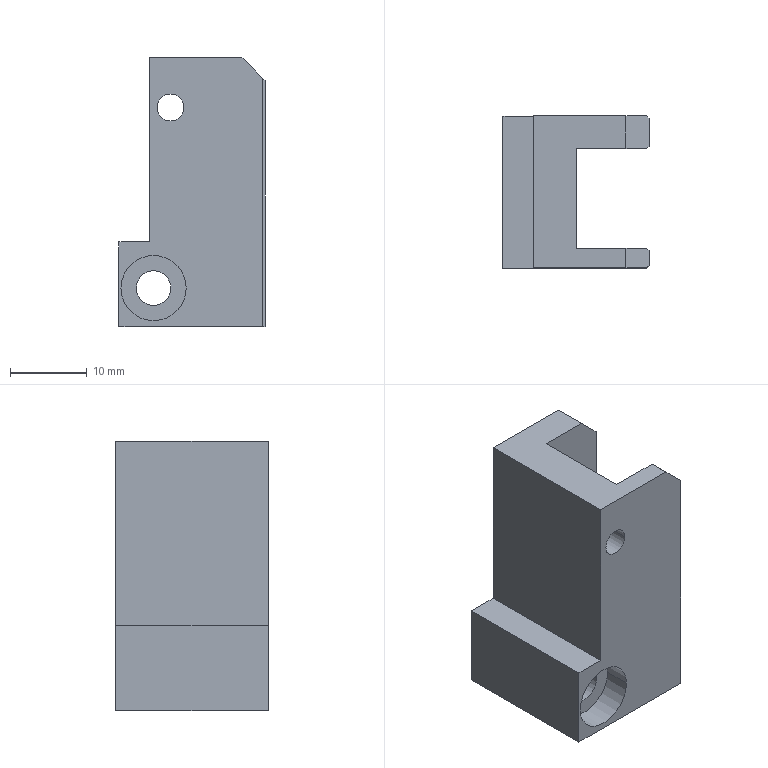Part | NX | 1 solid | 25 faces | box 19 x 19.788 x 35 mm | volume 6253 mm3 | plane 19 | cylinder 6 | commonest cylinder face diameters 3.5 x2 4.5 x2 8.5 x2
STEP:
#1=CARTESIAN_POINT('',(9.5,16.462,0.));
#2=VERTEX_POINT('',#1);
#3=CARTESIAN_POINT('',(18.7,16.462,0.));
#4=VERTEX_POINT('',#3);
#5=CARTESIAN_POINT('',(0.,16.462,0.));
#6=DIRECTION('',(1.,0.,0.));
#7=VECTOR('',#6,1000.);
#8=LINE('',#5,#7);
#9=EDGE_CURVE('',#2,#4,#8,.T.);
#10=ORIENTED_EDGE('',*,*,#9,.F.);
#11=CARTESIAN_POINT('',(9.5,3.462,0.));
#12=VERTEX_POINT('',#11);
#13=CARTESIAN_POINT('',(9.5,0.,0.));
#14=DIRECTION('',(0.,1.,0.));
#15=VECTOR('',#14,1000.);
#16=LINE('',#13,#15);
#17=EDGE_CURVE('',#12,#2,#16,.T.);
#18=ORIENTED_EDGE('',*,*,#17,.F.);
#19=CARTESIAN_POINT('',(18.7,3.462,0.));
#20=VERTEX_POINT('',#19);
#21=CARTESIAN_POINT('',(0.,3.462,0.));
#22=DIRECTION('',(-1.,0.,0.));
#23=VECTOR('',#22,1000.);
#24=LINE('',#21,#23);
#25=EDGE_CURVE('',#20,#12,#24,.T.);
#26=ORIENTED_EDGE('',*,*,#25,.F.);
#27=CARTESIAN_POINT('',(19.,3.162,0.));
#28=VERTEX_POINT('',#27);
#29=CARTESIAN_POINT('',(0.,22.162,0.));
#30=DIRECTION('',(0.7071,-0.7071,0.));
#31=VECTOR('',#30,1000.);
#32=LINE('',#29,#31);
#33=EDGE_CURVE('',#20,#28,#32,.T.);
#34=ORIENTED_EDGE('',*,*,#33,.T.);
#35=CARTESIAN_POINT('',(19.,1.212,0.));
#36=VERTEX_POINT('',#35);
#37=CARTESIAN_POINT('',(19.,0.,0.));
#38=DIRECTION('',(0.,-1.,0.));
#39=VECTOR('',#38,1000.);
#40=LINE('',#37,#39);
#41=EDGE_CURVE('',#28,#36,#40,.T.);
#42=ORIENTED_EDGE('',*,*,#41,.T.);
#43=CARTESIAN_POINT('',(18.7,0.912,0.));
#44=VERTEX_POINT('',#43);
#45=CARTESIAN_POINT('',(0.,-17.788,0.));
#46=DIRECTION('',(0.7071,0.7071,0.));
#47=VECTOR('',#46,1000.);
#48=LINE('',#45,#47);
#49=EDGE_CURVE('',#44,#36,#48,.T.);
#50=ORIENTED_EDGE('',*,*,#49,.F.);
#51=CARTESIAN_POINT('',(0.,0.912,0.));
#52=VERTEX_POINT('',#51);
#53=CARTESIAN_POINT('',(0.,0.912,0.));
#54=DIRECTION('',(-1.,0.,0.));
#55=VECTOR('',#54,1000.);
#56=LINE('',#53,#55);
#57=EDGE_CURVE('',#44,#52,#56,.T.);
#58=ORIENTED_EDGE('',*,*,#57,.T.);
#59=CARTESIAN_POINT('',(0.,20.7,0.));
#60=VERTEX_POINT('',#59);
#61=CARTESIAN_POINT('',(0.,0.,0.));
#62=DIRECTION('',(0.,-1.,0.));
#63=VECTOR('',#62,1000.);
#64=LINE('',#61,#63);
#65=EDGE_CURVE('',#60,#52,#64,.T.);
#66=ORIENTED_EDGE('',*,*,#65,.F.);
#67=CARTESIAN_POINT('',(18.7,20.7,0.));
#68=VERTEX_POINT('',#67);
#69=CARTESIAN_POINT('',(0.,20.7,0.));
#70=DIRECTION('',(1.,0.,0.));
#71=VECTOR('',#70,1000.);
#72=LINE('',#69,#71);
#73=EDGE_CURVE('',#60,#68,#72,.T.);
#74=ORIENTED_EDGE('',*,*,#73,.T.);
#75=CARTESIAN_POINT('',(19.,20.4,0.));
#76=VERTEX_POINT('',#75);
#77=CARTESIAN_POINT('',(39.4,0.,0.));
#78=DIRECTION('',(0.7071,-0.7071,0.));
#79=VECTOR('',#78,1000.);
#80=LINE('',#77,#79);
#81=EDGE_CURVE('',#68,#76,#80,.T.);
#82=ORIENTED_EDGE('',*,*,#81,.T.);
#83=CARTESIAN_POINT('',(19.,16.762,0.));
#84=VERTEX_POINT('',#83);
#85=CARTESIAN_POINT('',(19.,0.,0.));
#86=DIRECTION('',(0.,1.,0.));
#87=VECTOR('',#86,1000.);
#88=LINE('',#85,#87);
#89=EDGE_CURVE('',#84,#76,#88,.T.);
#90=ORIENTED_EDGE('',*,*,#89,.F.);
#91=CARTESIAN_POINT('',(2.238,0.,0.));
#92=DIRECTION('',(0.7071,0.7071,0.));
#93=VECTOR('',#92,1000.);
#94=LINE('',#91,#93);
#95=EDGE_CURVE('',#4,#84,#94,.T.);
#96=ORIENTED_EDGE('',*,*,#95,.F.);
#97=EDGE_LOOP('',(#10,#18,#26,#34,#42,#50,#58,#66,#74,#82,#90,#96));
#98=FACE_BOUND('',#97,.T.);
#99=CARTESIAN_POINT('',(0.,0.,0.));
#100=DIRECTION('',(0.,0.,1.));
#101=DIRECTION('',(1.,0.,0.));
#102=AXIS2_PLACEMENT_3D('',#99,#100,#101);
#103=PLANE('',#102);
#104=ADVANCED_FACE('',(#98),#103,.F.);
#105=CARTESIAN_POINT('',(18.7,16.462,32.3));
#106=VERTEX_POINT('',#105);
#107=CARTESIAN_POINT('',(18.7,16.462,0.));
#108=DIRECTION('',(0.,0.,-1.));
#109=VECTOR('',#108,1000.);
#110=LINE('',#107,#109);
#111=EDGE_CURVE('',#106,#4,#110,.T.);
#112=ORIENTED_EDGE('',*,*,#111,.F.);
#113=CARTESIAN_POINT('',(16.,16.462,35.));
#114=VERTEX_POINT('',#113);
#115=CARTESIAN_POINT('',(51.,16.462,0.));
#116=DIRECTION('',(-0.7071,0.,0.7071));
#117=VECTOR('',#116,1000.);
#118=LINE('',#115,#117);
#119=EDGE_CURVE('',#106,#114,#118,.T.);
#120=ORIENTED_EDGE('',*,*,#119,.T.);
#121=CARTESIAN_POINT('',(9.5,16.462,35.));
#122=VERTEX_POINT('',#121);
#123=CARTESIAN_POINT('',(0.,16.462,35.));
#124=DIRECTION('',(1.,0.,0.));
#125=VECTOR('',#124,1000.);
#126=LINE('',#123,#125);
#127=EDGE_CURVE('',#122,#114,#126,.T.);
#128=ORIENTED_EDGE('',*,*,#127,.F.);
#129=CARTESIAN_POINT('',(9.5,16.462,0.));
#130=DIRECTION('',(0.,0.,1.));
#131=VECTOR('',#130,1000.);
#132=LINE('',#129,#131);
#133=EDGE_CURVE('',#2,#122,#132,.T.);
#134=ORIENTED_EDGE('',*,*,#133,.F.);
#135=ORIENTED_EDGE('',*,*,#9,.T.);
#136=EDGE_LOOP('',(#112,#120,#128,#134,#135));
#137=FACE_BOUND('',#136,.T.);
#138=CARTESIAN_POINT('',(19.,16.462,35.));
#139=DIRECTION('',(0.,1.,0.));
#140=DIRECTION('',(1.,0.,0.));
#141=AXIS2_PLACEMENT_3D('',#138,#139,#140);
#142=PLANE('',#141);
#143=ADVANCED_FACE('',(#137),#142,.F.);
#144=ORIENTED_EDGE('',*,*,#17,.T.);
#145=ORIENTED_EDGE('',*,*,#133,.T.);
#146=CARTESIAN_POINT('',(9.5,3.462,35.));
#147=VERTEX_POINT('',#146);
#148=CARTESIAN_POINT('',(9.5,0.,35.));
#149=DIRECTION('',(0.,1.,0.));
#150=VECTOR('',#149,1000.);
#151=LINE('',#148,#150);
#152=EDGE_CURVE('',#147,#122,#151,.T.);
#153=ORIENTED_EDGE('',*,*,#152,.F.);
#154=CARTESIAN_POINT('',(9.5,3.462,0.));
#155=DIRECTION('',(0.,0.,1.));
#156=VECTOR('',#155,1000.);
#157=LINE('',#154,#156);
#158=EDGE_CURVE('',#12,#147,#157,.T.);
#159=ORIENTED_EDGE('',*,*,#158,.F.);
#160=EDGE_LOOP('',(#144,#145,#153,#159));
#161=FACE_BOUND('',#160,.T.);
#162=CARTESIAN_POINT('',(9.5,16.95,35.));
#163=DIRECTION('',(-1.,0.,0.));
#164=DIRECTION('',(0.,0.,1.));
#165=AXIS2_PLACEMENT_3D('',#162,#163,#164);
#166=PLANE('',#165);
#167=ADVANCED_FACE('',(#161),#166,.F.);
#168=CARTESIAN_POINT('',(18.7,3.462,32.3));
#169=VERTEX_POINT('',#168);
#170=CARTESIAN_POINT('',(18.7,3.462,0.));
#171=DIRECTION('',(0.,0.,-1.));
#172=VECTOR('',#171,1000.);
#173=LINE('',#170,#172);
#174=EDGE_CURVE('',#169,#20,#173,.T.);
#175=ORIENTED_EDGE('',*,*,#174,.T.);
#176=ORIENTED_EDGE('',*,*,#25,.T.);
#177=ORIENTED_EDGE('',*,*,#158,.T.);
#178=CARTESIAN_POINT('',(16.,3.462,35.));
#179=VERTEX_POINT('',#178);
#180=CARTESIAN_POINT('',(0.,3.462,35.));
#181=DIRECTION('',(-1.,0.,0.));
#182=VECTOR('',#181,1000.);
#183=LINE('',#180,#182);
#184=EDGE_CURVE('',#179,#147,#183,.T.);
#185=ORIENTED_EDGE('',*,*,#184,.F.);
#186=CARTESIAN_POINT('',(51.,3.462,0.));
#187=DIRECTION('',(0.7071,0.,-0.7071));
#188=VECTOR('',#187,1000.);
#189=LINE('',#186,#188);
#190=EDGE_CURVE('',#179,#169,#189,.T.);
#191=ORIENTED_EDGE('',*,*,#190,.T.);
#192=EDGE_LOOP('',(#175,#176,#177,#185,#191));
#193=FACE_BOUND('',#192,.T.);
#194=CARTESIAN_POINT('',(9.5,3.462,35.));
#195=DIRECTION('',(0.,-1.,0.));
#196=DIRECTION('',(0.,0.,-1.));
#197=AXIS2_PLACEMENT_3D('',#194,#195,#196);
#198=PLANE('',#197);
#199=ADVANCED_FACE('',(#193),#198,.F.);
#200=CARTESIAN_POINT('',(19.,3.162,32.));
#201=VERTEX_POINT('',#200);
#202=CARTESIAN_POINT('',(19.,3.162,0.));
#203=DIRECTION('',(0.,0.,-1.));
#204=VECTOR('',#203,1000.);
#205=LINE('',#202,#204);
#206=EDGE_CURVE('',#201,#28,#205,.T.);
#207=ORIENTED_EDGE('',*,*,#206,.F.);
#208=CARTESIAN_POINT('',(19.,1.212,32.));
#209=VERTEX_POINT('',#208);
#210=CARTESIAN_POINT('',(19.,0.,32.));
#211=DIRECTION('',(0.,1.,0.));
#212=VECTOR('',#211,1000.);
#213=LINE('',#210,#212);
#214=EDGE_CURVE('',#209,#201,#213,.T.);
#215=ORIENTED_EDGE('',*,*,#214,.F.);
#216=CARTESIAN_POINT('',(19.,1.212,0.));
#217=DIRECTION('',(0.,0.,-1.));
#218=VECTOR('',#217,1000.);
#219=LINE('',#216,#218);
#220=EDGE_CURVE('',#209,#36,#219,.T.);
#221=ORIENTED_EDGE('',*,*,#220,.T.);
#222=ORIENTED_EDGE('',*,*,#41,.F.);
#223=EDGE_LOOP('',(#207,#215,#221,#222));
#224=FACE_BOUND('',#223,.T.);
#225=CARTESIAN_POINT('',(19.,0.,0.));
#226=DIRECTION('',(1.,0.,0.));
#227=DIRECTION('',(0.,1.,0.));
#228=AXIS2_PLACEMENT_3D('',#225,#226,#227);
#229=PLANE('',#228);
#230=ADVANCED_FACE('',(#224),#229,.T.);
#231=CARTESIAN_POINT('',(0.25,4.4,5.));
#232=VERTEX_POINT('',#231);
#233=CARTESIAN_POINT('',(8.75,4.4,5.));
#234=VERTEX_POINT('',#233);
#235=CARTESIAN_POINT('',(4.5,4.4,5.));
#236=DIRECTION('',(0.,-1.,0.));
#237=DIRECTION('',(-1.,0.,0.));
#238=AXIS2_PLACEMENT_3D('',#235,#236,#237);
#239=CIRCLE('',#238,4.25);
#240=EDGE_CURVE('',#232,#234,#239,.T.);
#241=ORIENTED_EDGE('',*,*,#240,.T.);
#242=CARTESIAN_POINT('',(4.5,4.4,5.));
#243=DIRECTION('',(0.,-1.,0.));
#244=DIRECTION('',(-1.,0.,0.));
#245=AXIS2_PLACEMENT_3D('',#242,#243,#244);
#246=CIRCLE('',#245,4.25);
#247=EDGE_CURVE('',#234,#232,#246,.T.);
#248=ORIENTED_EDGE('',*,*,#247,.T.);
#249=EDGE_LOOP('',(#241,#248));
#250=FACE_BOUND('',#249,.T.);
#251=CARTESIAN_POINT('',(2.25,4.4,5.));
#252=VERTEX_POINT('',#251);
#253=CARTESIAN_POINT('',(6.75,4.4,5.));
#254=VERTEX_POINT('',#253);
#255=CARTESIAN_POINT('',(4.5,4.4,5.));
#256=DIRECTION('',(0.,-1.,0.));
#257=DIRECTION('',(1.,0.,0.));
#258=AXIS2_PLACEMENT_3D('',#255,#256,#257);
#259=CIRCLE('',#258,2.25);
#260=EDGE_CURVE('',#252,#254,#259,.T.);
#261=ORIENTED_EDGE('',*,*,#260,.F.);
#262=CARTESIAN_POINT('',(4.5,4.4,5.));
#263=DIRECTION('',(0.,-1.,0.));
#264=DIRECTION('',(1.,0.,0.));
#265=AXIS2_PLACEMENT_3D('',#262,#263,#264);
#266=CIRCLE('',#265,2.25);
#267=EDGE_CURVE('',#254,#252,#266,.T.);
#268=ORIENTED_EDGE('',*,*,#267,.F.);
#269=EDGE_LOOP('',(#261,#268));
#270=FACE_BOUND('',#269,.T.);
#271=CARTESIAN_POINT('',(9.199,4.4,2.964));
#272=DIRECTION('',(0.,-1.,0.));
#273=DIRECTION('',(0.,0.,-1.));
#274=AXIS2_PLACEMENT_3D('',#271,#272,#273);
#275=PLANE('',#274);
#276=ADVANCED_FACE('',(#250,#270),#275,.T.);
#277=CARTESIAN_POINT('',(4.,20.7,35.));
#278=VERTEX_POINT('',#277);
#279=CARTESIAN_POINT('',(4.,0.912,35.));
#280=VERTEX_POINT('',#279);
#281=CARTESIAN_POINT('',(4.,0.,35.));
#282=DIRECTION('',(0.,-1.,0.));
#283=VECTOR('',#282,1000.);
#284=LINE('',#281,#283);
#285=EDGE_CURVE('',#278,#280,#284,.T.);
#286=ORIENTED_EDGE('',*,*,#285,.F.);
#287=CARTESIAN_POINT('',(4.,20.7,11.));
#288=VERTEX_POINT('',#287);
#289=CARTESIAN_POINT('',(4.,20.7,0.));
#290=DIRECTION('',(0.,0.,-1.));
#291=VECTOR('',#290,1000.);
#292=LINE('',#289,#291);
#293=EDGE_CURVE('',#278,#288,#292,.T.);
#294=ORIENTED_EDGE('',*,*,#293,.T.);
#295=CARTESIAN_POINT('',(4.,0.912,11.));
#296=VERTEX_POINT('',#295);
#297=CARTESIAN_POINT('',(4.,0.,11.));
#298=DIRECTION('',(0.,1.,0.));
#299=VECTOR('',#298,1000.);
#300=LINE('',#297,#299);
#301=EDGE_CURVE('',#296,#288,#300,.T.);
#302=ORIENTED_EDGE('',*,*,#301,.F.);
#303=CARTESIAN_POINT('',(4.,0.912,0.));
#304=DIRECTION('',(0.,0.,1.));
#305=VECTOR('',#304,1000.);
#306=LINE('',#303,#305);
#307=EDGE_CURVE('',#296,#280,#306,.T.);
#308=ORIENTED_EDGE('',*,*,#307,.T.);
#309=EDGE_LOOP('',(#286,#294,#302,#308));
#310=FACE_BOUND('',#309,.T.);
#311=CARTESIAN_POINT('',(4.,20.5,35.));
#312=DIRECTION('',(1.,0.,0.));
#313=DIRECTION('',(0.,1.,0.));
#314=AXIS2_PLACEMENT_3D('',#311,#312,#313);
#315=PLANE('',#314);
#316=ADVANCED_FACE('',(#310),#315,.F.);
#317=ORIENTED_EDGE('',*,*,#285,.T.);
#318=CARTESIAN_POINT('',(16.,0.912,35.));
#319=VERTEX_POINT('',#318);
#320=CARTESIAN_POINT('',(0.,0.912,35.));
#321=DIRECTION('',(-1.,0.,0.));
#322=VECTOR('',#321,1000.);
#323=LINE('',#320,#322);
#324=EDGE_CURVE('',#319,#280,#323,.T.);
#325=ORIENTED_EDGE('',*,*,#324,.F.);
#326=CARTESIAN_POINT('',(16.,0.,35.));
#327=DIRECTION('',(0.,1.,0.));
#328=VECTOR('',#327,1000.);
#329=LINE('',#326,#328);
#330=EDGE_CURVE('',#319,#179,#329,.T.);
#331=ORIENTED_EDGE('',*,*,#330,.T.);
#332=ORIENTED_EDGE('',*,*,#184,.T.);
#333=ORIENTED_EDGE('',*,*,#152,.T.);
#334=ORIENTED_EDGE('',*,*,#127,.T.);
#335=CARTESIAN_POINT('',(16.,20.7,35.));
#336=VERTEX_POINT('',#335);
#337=CARTESIAN_POINT('',(16.,0.,35.));
#338=DIRECTION('',(0.,-1.,0.));
#339=VECTOR('',#338,1000.);
#340=LINE('',#337,#339);
#341=EDGE_CURVE('',#336,#114,#340,.T.);
#342=ORIENTED_EDGE('',*,*,#341,.F.);
#343=CARTESIAN_POINT('',(0.,20.7,35.));
#344=DIRECTION('',(1.,0.,0.));
#345=VECTOR('',#344,1000.);
#346=LINE('',#343,#345);
#347=EDGE_CURVE('',#278,#336,#346,.T.);
#348=ORIENTED_EDGE('',*,*,#347,.F.);
#349=EDGE_LOOP('',(#317,#325,#331,#332,#333,#334,#342,#348));
#350=FACE_BOUND('',#349,.T.);
#351=CARTESIAN_POINT('',(0.,0.,35.));
#352=DIRECTION('',(0.,0.,1.));
#353=DIRECTION('',(1.,0.,0.));
#354=AXIS2_PLACEMENT_3D('',#351,#352,#353);
#355=PLANE('',#354);
#356=ADVANCED_FACE('',(#350),#355,.T.);
#357=CARTESIAN_POINT('',(18.7,0.912,32.3));
#358=VERTEX_POINT('',#357);
#359=CARTESIAN_POINT('',(18.7,0.912,0.));
#360=DIRECTION('',(0.,0.,1.));
#361=VECTOR('',#360,1000.);
#362=LINE('',#359,#361);
#363=EDGE_CURVE('',#44,#358,#362,.T.);
#364=ORIENTED_EDGE('',*,*,#363,.T.);
#365=CARTESIAN_POINT('',(51.,0.912,0.));
#366=DIRECTION('',(0.7071,0.,-0.7071));
#367=VECTOR('',#366,1000.);
#368=LINE('',#365,#367);
#369=EDGE_CURVE('',#319,#358,#368,.T.);
#370=ORIENTED_EDGE('',*,*,#369,.F.);
#371=ORIENTED_EDGE('',*,*,#324,.T.);
#372=ORIENTED_EDGE('',*,*,#307,.F.);
#373=CARTESIAN_POINT('',(0.,0.912,11.));
#374=VERTEX_POINT('',#373);
#375=CARTESIAN_POINT('',(0.,0.912,11.));
#376=DIRECTION('',(1.,0.,0.));
#377=VECTOR('',#376,1000.);
#378=LINE('',#375,#377);
#379=EDGE_CURVE('',#374,#296,#378,.T.);
#380=ORIENTED_EDGE('',*,*,#379,.F.);
#381=CARTESIAN_POINT('',(0.,0.912,0.));
#382=DIRECTION('',(0.,0.,-1.));
#383=VECTOR('',#382,1000.);
#384=LINE('',#381,#383);
#385=EDGE_CURVE('',#374,#52,#384,.T.);
#386=ORIENTED_EDGE('',*,*,#385,.T.);
#387=ORIENTED_EDGE('',*,*,#57,.F.);
#388=EDGE_LOOP('',(#364,#370,#371,#372,#380,#386,#387));
#389=FACE_BOUND('',#388,.T.);
#390=CARTESIAN_POINT('',(8.45,0.912,28.5));
#391=VERTEX_POINT('',#390);
#392=CARTESIAN_POINT('',(4.95,0.912,28.5));
#393=VERTEX_POINT('',#392);
#394=CARTESIAN_POINT('',(6.7,0.912,28.5));
#395=DIRECTION('',(0.,-1.,0.));
#396=DIRECTION('',(1.,0.,0.));
#397=AXIS2_PLACEMENT_3D('',#394,#395,#396);
#398=CIRCLE('',#397,1.75);
#399=EDGE_CURVE('',#391,#393,#398,.T.);
#400=ORIENTED_EDGE('',*,*,#399,.F.);
#401=CARTESIAN_POINT('',(6.7,0.912,28.5));
#402=DIRECTION('',(0.,-1.,0.));
#403=DIRECTION('',(1.,0.,0.));
#404=AXIS2_PLACEMENT_3D('',#401,#402,#403);
#405=CIRCLE('',#404,1.75);
#406=EDGE_CURVE('',#393,#391,#405,.T.);
#407=ORIENTED_EDGE('',*,*,#406,.F.);
#408=EDGE_LOOP('',(#400,#407));
#409=FACE_BOUND('',#408,.T.);
#410=CARTESIAN_POINT('',(0.25,0.912,5.));
#411=VERTEX_POINT('',#410);
#412=CARTESIAN_POINT('',(8.75,0.912,5.));
#413=VERTEX_POINT('',#412);
#414=CARTESIAN_POINT('',(4.5,0.912,5.));
#415=DIRECTION('',(0.,-1.,0.));
#416=DIRECTION('',(-1.,0.,0.));
#417=AXIS2_PLACEMENT_3D('',#414,#415,#416);
#418=CIRCLE('',#417,4.25);
#419=EDGE_CURVE('',#411,#413,#418,.T.);
#420=ORIENTED_EDGE('',*,*,#419,.F.);
#421=CARTESIAN_POINT('',(4.5,0.912,5.));
#422=DIRECTION('',(0.,-1.,0.));
#423=DIRECTION('',(-1.,0.,0.));
#424=AXIS2_PLACEMENT_3D('',#421,#422,#423);
#425=CIRCLE('',#424,4.25);
#426=EDGE_CURVE('',#413,#411,#425,.T.);
#427=ORIENTED_EDGE('',*,*,#426,.F.);
#428=EDGE_LOOP('',(#420,#427));
#429=FACE_BOUND('',#428,.T.);
#430=CARTESIAN_POINT('',(0.,0.912,0.));
#431=DIRECTION('',(0.,-1.,0.));
#432=DIRECTION('',(0.,0.,-1.));
#433=AXIS2_PLACEMENT_3D('',#430,#431,#432);
#434=PLANE('',#433);
#435=ADVANCED_FACE('',(#389,#409,#429),#434,.T.);
#436=ORIENTED_EDGE('',*,*,#379,.T.);
#437=ORIENTED_EDGE('',*,*,#301,.T.);
#438=CARTESIAN_POINT('',(0.,20.7,11.));
#439=VERTEX_POINT('',#438);
#440=CARTESIAN_POINT('',(0.,20.7,11.));
#441=DIRECTION('',(-1.,0.,0.));
#442=VECTOR('',#441,1000.);
#443=LINE('',#440,#442);
#444=EDGE_CURVE('',#288,#439,#443,.T.);
#445=ORIENTED_EDGE('',*,*,#444,.T.);
#446=CARTESIAN_POINT('',(0.,0.,11.));
#447=DIRECTION('',(0.,-1.,0.));
#448=VECTOR('',#447,1000.);
#449=LINE('',#446,#448);
#450=EDGE_CURVE('',#439,#374,#449,.T.);
#451=ORIENTED_EDGE('',*,*,#450,.T.);
#452=EDGE_LOOP('',(#436,#437,#445,#451));
#453=FACE_BOUND('',#452,.T.);
#454=CARTESIAN_POINT('',(4.,20.5,11.));
#455=DIRECTION('',(0.,0.,-1.));
#456=DIRECTION('',(0.,-1.,0.));
#457=AXIS2_PLACEMENT_3D('',#454,#455,#456);
#458=PLANE('',#457);
#459=ADVANCED_FACE('',(#453),#458,.F.);
#460=ORIENTED_EDGE('',*,*,#450,.F.);
#461=CARTESIAN_POINT('',(0.,20.7,0.));
#462=DIRECTION('',(0.,0.,1.));
#463=VECTOR('',#462,1000.);
#464=LINE('',#461,#463);
#465=EDGE_CURVE('',#60,#439,#464,.T.);
#466=ORIENTED_EDGE('',*,*,#465,.F.);
#467=ORIENTED_EDGE('',*,*,#65,.T.);
#468=ORIENTED_EDGE('',*,*,#385,.F.);
#469=EDGE_LOOP('',(#460,#466,#467,#468));
#470=FACE_BOUND('',#469,.T.);
#471=CARTESIAN_POINT('',(0.,20.5,0.));
#472=DIRECTION('',(-1.,0.,0.));
#473=DIRECTION('',(0.,0.,1.));
#474=AXIS2_PLACEMENT_3D('',#471,#472,#473);
#475=PLANE('',#474);
#476=ADVANCED_FACE('',(#470),#475,.T.);
#477=CARTESIAN_POINT('',(19.,16.762,32.));
#478=VERTEX_POINT('',#477);
#479=CARTESIAN_POINT('',(19.,16.762,0.));
#480=DIRECTION('',(0.,0.,-1.));
#481=VECTOR('',#480,1000.);
#482=LINE('',#479,#481);
#483=EDGE_CURVE('',#478,#84,#482,.T.);
#484=ORIENTED_EDGE('',*,*,#483,.T.);
#485=ORIENTED_EDGE('',*,*,#89,.T.);
#486=CARTESIAN_POINT('',(19.,20.4,32.));
#487=VERTEX_POINT('',#486);
#488=CARTESIAN_POINT('',(19.,20.4,0.));
#489=DIRECTION('',(0.,0.,-1.));
#490=VECTOR('',#489,1000.);
#491=LINE('',#488,#490);
#492=EDGE_CURVE('',#487,#76,#491,.T.);
#493=ORIENTED_EDGE('',*,*,#492,.F.);
#494=CARTESIAN_POINT('',(19.,0.,32.));
#495=DIRECTION('',(0.,-1.,0.));
#496=VECTOR('',#495,1000.);
#497=LINE('',#494,#496);
#498=EDGE_CURVE('',#487,#478,#497,.T.);
#499=ORIENTED_EDGE('',*,*,#498,.T.);
#500=EDGE_LOOP('',(#484,#485,#493,#499));
#501=FACE_BOUND('',#500,.T.);
#502=CARTESIAN_POINT('',(19.,0.,0.));
#503=DIRECTION('',(1.,0.,0.));
#504=DIRECTION('',(0.,1.,0.));
#505=AXIS2_PLACEMENT_3D('',#502,#503,#504);
#506=PLANE('',#505);
#507=ADVANCED_FACE('',(#501),#506,.T.);
#508=ORIENTED_EDGE('',*,*,#341,.T.);
#509=ORIENTED_EDGE('',*,*,#119,.F.);
#510=CARTESIAN_POINT('',(51.,48.762,0.));
#511=DIRECTION('',(-0.5774,-0.5774,0.5774));
#512=VECTOR('',#511,1000.);
#513=LINE('',#510,#512);
#514=EDGE_CURVE('',#478,#106,#513,.T.);
#515=ORIENTED_EDGE('',*,*,#514,.F.);
#516=ORIENTED_EDGE('',*,*,#498,.F.);
#517=CARTESIAN_POINT('',(18.7,20.7,32.3));
#518=VERTEX_POINT('',#517);
#519=CARTESIAN_POINT('',(51.,-11.6,0.));
#520=DIRECTION('',(-0.5774,0.5774,0.5774));
#521=VECTOR('',#520,1000.);
#522=LINE('',#519,#521);
#523=EDGE_CURVE('',#487,#518,#522,.T.);
#524=ORIENTED_EDGE('',*,*,#523,.T.);
#525=CARTESIAN_POINT('',(51.,20.7,0.));
#526=DIRECTION('',(-0.7071,0.,0.7071));
#527=VECTOR('',#526,1000.);
#528=LINE('',#525,#527);
#529=EDGE_CURVE('',#518,#336,#528,.T.);
#530=ORIENTED_EDGE('',*,*,#529,.T.);
#531=EDGE_LOOP('',(#508,#509,#515,#516,#524,#530));
#532=FACE_BOUND('',#531,.T.);
#533=CARTESIAN_POINT('',(16.,16.95,35.));
#534=DIRECTION('',(-0.7071,0.,-0.7071));
#535=DIRECTION('',(-0.7071,0.,0.7071));
#536=AXIS2_PLACEMENT_3D('',#533,#534,#535);
#537=PLANE('',#536);
#538=ADVANCED_FACE('',(#532),#537,.F.);
#539=CARTESIAN_POINT('',(8.45,20.7,28.5));
#540=VERTEX_POINT('',#539);
#541=CARTESIAN_POINT('',(4.95,20.7,28.5));
#542=VERTEX_POINT('',#541);
#543=CARTESIAN_POINT('',(6.7,20.7,28.5));
#544=DIRECTION('',(0.,-1.,0.));
#545=DIRECTION('',(1.,0.,0.));
#546=AXIS2_PLACEMENT_3D('',#543,#544,#545);
#547=CIRCLE('',#546,1.75);
#548=EDGE_CURVE('',#540,#542,#547,.T.);
#549=ORIENTED_EDGE('',*,*,#548,.F.);
#550=CARTESIAN_POINT('',(8.45,20.5,28.5));
#551=DIRECTION('',(0.,-1.,0.));
#552=VECTOR('',#551,1000.);
#553=LINE('',#550,#552);
#554=EDGE_CURVE('',#540,#391,#553,.T.);
#555=ORIENTED_EDGE('',*,*,#554,.T.);
#556=ORIENTED_EDGE('',*,*,#399,.T.);
#557=CARTESIAN_POINT('',(4.95,20.5,28.5));
#558=DIRECTION('',(0.,-1.,0.));
#559=VECTOR('',#558,1000.);
#560=LINE('',#557,#559);
#561=EDGE_CURVE('',#542,#393,#560,.T.);
#562=ORIENTED_EDGE('',*,*,#561,.F.);
#563=EDGE_LOOP('',(#549,#555,#556,#562));
#564=FACE_BOUND('',#563,.T.);
#565=CARTESIAN_POINT('',(6.7,20.5,28.5));
#566=DIRECTION('',(0.,-1.,0.));
#567=DIRECTION('',(1.,0.,0.));
#568=AXIS2_PLACEMENT_3D('',#565,#566,#567);
#569=CYLINDRICAL_SURFACE('',#568,1.75);
#570=ADVANCED_FACE('',(#564),#569,.F.);
#571=ORIENTED_EDGE('',*,*,#330,.F.);
#572=ORIENTED_EDGE('',*,*,#369,.T.);
#573=CARTESIAN_POINT('',(51.,33.212,0.));
#574=DIRECTION('',(-0.5774,-0.5774,0.5774));
#575=VECTOR('',#574,1000.);
#576=LINE('',#573,#575);
#577=EDGE_CURVE('',#209,#358,#576,.T.);
#578=ORIENTED_EDGE('',*,*,#577,.F.);
#579=ORIENTED_EDGE('',*,*,#214,.T.);
#580=CARTESIAN_POINT('',(51.,-28.838,0.));
#581=DIRECTION('',(-0.5774,0.5774,0.5774));
#582=VECTOR('',#581,1000.);
#583=LINE('',#580,#582);
#584=EDGE_CURVE('',#201,#169,#583,.T.);
#585=ORIENTED_EDGE('',*,*,#584,.T.);
#586=ORIENTED_EDGE('',*,*,#190,.F.);
#587=EDGE_LOOP('',(#571,#572,#578,#579,#585,#586));
#588=FACE_BOUND('',#587,.T.);
#589=CARTESIAN_POINT('',(16.,0.,35.));
#590=DIRECTION('',(-0.7071,0.,-0.7071));
#591=DIRECTION('',(-0.7071,0.,0.7071));
#592=AXIS2_PLACEMENT_3D('',#589,#590,#591);
#593=PLANE('',#592);
#594=ADVANCED_FACE('',(#588),#593,.F.);
#595=CARTESIAN_POINT('',(6.75,20.7,5.));
#596=VERTEX_POINT('',#595);
#597=CARTESIAN_POINT('',(2.25,20.7,5.));
#598=VERTEX_POINT('',#597);
#599=CARTESIAN_POINT('',(4.5,20.7,5.));
#600=DIRECTION('',(0.,-1.,0.));
#601=DIRECTION('',(1.,0.,0.));
#602=AXIS2_PLACEMENT_3D('',#599,#600,#601);
#603=CIRCLE('',#602,2.25);
#604=EDGE_CURVE('',#596,#598,#603,.T.);
#605=ORIENTED_EDGE('',*,*,#604,.F.);
#606=CARTESIAN_POINT('',(6.75,20.5,5.));
#607=DIRECTION('',(0.,-1.,0.));
#608=VECTOR('',#607,1000.);
#609=LINE('',#606,#608);
#610=EDGE_CURVE('',#596,#254,#609,.T.);
#611=ORIENTED_EDGE('',*,*,#610,.T.);
#612=ORIENTED_EDGE('',*,*,#267,.T.);
#613=CARTESIAN_POINT('',(2.25,20.5,5.));
#614=DIRECTION('',(0.,-1.,0.));
#615=VECTOR('',#614,1000.);
#616=LINE('',#613,#615);
#617=EDGE_CURVE('',#598,#252,#616,.T.);
#618=ORIENTED_EDGE('',*,*,#617,.F.);
#619=EDGE_LOOP('',(#605,#611,#612,#618));
#620=FACE_BOUND('',#619,.T.);
#621=CARTESIAN_POINT('',(4.5,20.5,5.));
#622=DIRECTION('',(0.,-1.,0.));
#623=DIRECTION('',(1.,0.,0.));
#624=AXIS2_PLACEMENT_3D('',#621,#622,#623);
#625=CYLINDRICAL_SURFACE('',#624,2.25);
#626=ADVANCED_FACE('',(#620),#625,.F.);
#627=ORIENTED_EDGE('',*,*,#419,.T.);
#628=CARTESIAN_POINT('',(8.75,0.9,5.));
#629=DIRECTION('',(0.,-1.,0.));
#630=VECTOR('',#629,1000.);
#631=LINE('',#628,#630);
#632=EDGE_CURVE('',#413,#234,#631,.F.);
#633=ORIENTED_EDGE('',*,*,#632,.T.);
#634=ORIENTED_EDGE('',*,*,#240,.F.);
#635=CARTESIAN_POINT('',(0.25,0.9,5.));
#636=DIRECTION('',(0.,-1.,0.));
#637=VECTOR('',#636,1000.);
#638=LINE('',#635,#637);
#639=EDGE_CURVE('',#411,#232,#638,.F.);
#640=ORIENTED_EDGE('',*,*,#639,.F.);
#641=EDGE_LOOP('',(#627,#633,#634,#640));
#642=FACE_BOUND('',#641,.T.);
#643=CARTESIAN_POINT('',(4.5,0.9,5.));
#644=DIRECTION('',(0.,-1.,0.));
#645=DIRECTION('',(-1.,0.,0.));
#646=AXIS2_PLACEMENT_3D('',#643,#644,#645);
#647=CYLINDRICAL_SURFACE('',#646,4.25);
#648=ADVANCED_FACE('',(#642),#647,.F.);
#649=CARTESIAN_POINT('',(18.7,20.7,0.));
#650=DIRECTION('',(0.,0.,1.));
#651=VECTOR('',#650,1000.);
#652=LINE('',#649,#651);
#653=EDGE_CURVE('',#68,#518,#652,.T.);
#654=ORIENTED_EDGE('',*,*,#653,.F.);
#655=ORIENTED_EDGE('',*,*,#73,.F.);
#656=ORIENTED_EDGE('',*,*,#465,.T.);
#657=ORIENTED_EDGE('',*,*,#444,.F.);
#658=ORIENTED_EDGE('',*,*,#293,.F.);
#659=ORIENTED_EDGE('',*,*,#347,.T.);
#660=ORIENTED_EDGE('',*,*,#529,.F.);
#661=EDGE_LOOP('',(#654,#655,#656,#657,#658,#659,#660));
#662=FACE_BOUND('',#661,.T.);
#663=ORIENTED_EDGE('',*,*,#548,.T.);
#664=CARTESIAN_POINT('',(6.7,20.7,28.5));
#665=DIRECTION('',(0.,-1.,0.));
#666=DIRECTION('',(1.,0.,0.));
#667=AXIS2_PLACEMENT_3D('',#664,#665,#666);
#668=CIRCLE('',#667,1.75);
#669=EDGE_CURVE('',#542,#540,#668,.T.);
#670=ORIENTED_EDGE('',*,*,#669,.T.);
#671=EDGE_LOOP('',(#663,#670));
#672=FACE_BOUND('',#671,.T.);
#673=ORIENTED_EDGE('',*,*,#604,.T.);
#674=CARTESIAN_POINT('',(4.5,20.7,5.));
#675=DIRECTION('',(0.,-1.,0.));
#676=DIRECTION('',(1.,0.,0.));
#677=AXIS2_PLACEMENT_3D('',#674,#675,#676);
#678=CIRCLE('',#677,2.25);
#679=EDGE_CURVE('',#598,#596,#678,.T.);
#680=ORIENTED_EDGE('',*,*,#679,.T.);
#681=EDGE_LOOP('',(#673,#680));
#682=FACE_BOUND('',#681,.T.);
#683=CARTESIAN_POINT('',(19.,20.7,0.));
#684=DIRECTION('',(0.,1.,0.));
#685=DIRECTION('',(1.,0.,0.));
#686=AXIS2_PLACEMENT_3D('',#683,#684,#685);
#687=PLANE('',#686);
#688=ADVANCED_FACE('',(#662,#672,#682),#687,.T.);
#689=ORIENTED_EDGE('',*,*,#111,.T.);
#690=ORIENTED_EDGE('',*,*,#95,.T.);
#691=ORIENTED_EDGE('',*,*,#483,.F.);
#692=ORIENTED_EDGE('',*,*,#514,.T.);
#693=EDGE_LOOP('',(#689,#690,#691,#692));
#694=FACE_BOUND('',#693,.T.);
#695=CARTESIAN_POINT('',(18.85,16.612,16.));
#696=DIRECTION('',(-0.7071,0.7071,0.));
#697=DIRECTION('',(0.,0.,1.));
#698=AXIS2_PLACEMENT_3D('',#695,#696,#697);
#699=PLANE('',#698);
#700=ADVANCED_FACE('',(#694),#699,.F.);
#701=ORIENTED_EDGE('',*,*,#363,.F.);
#702=ORIENTED_EDGE('',*,*,#49,.T.);
#703=ORIENTED_EDGE('',*,*,#220,.F.);
#704=ORIENTED_EDGE('',*,*,#577,.T.);
#705=EDGE_LOOP('',(#701,#702,#703,#704));
#706=FACE_BOUND('',#705,.T.);
#707=CARTESIAN_POINT('',(18.85,1.062,16.));
#708=DIRECTION('',(-0.7071,0.7071,0.));
#709=DIRECTION('',(0.,0.,1.));
#710=AXIS2_PLACEMENT_3D('',#707,#708,#709);
#711=PLANE('',#710);
#712=ADVANCED_FACE('',(#706),#711,.F.);
#713=ORIENTED_EDGE('',*,*,#174,.F.);
#714=ORIENTED_EDGE('',*,*,#584,.F.);
#715=ORIENTED_EDGE('',*,*,#206,.T.);
#716=ORIENTED_EDGE('',*,*,#33,.F.);
#717=EDGE_LOOP('',(#713,#714,#715,#716));
#718=FACE_BOUND('',#717,.T.);
#719=CARTESIAN_POINT('',(18.85,3.312,16.));
#720=DIRECTION('',(0.7071,0.7071,0.));
#721=DIRECTION('',(0.,0.,-1.));
#722=AXIS2_PLACEMENT_3D('',#719,#720,#721);
#723=PLANE('',#722);
#724=ADVANCED_FACE('',(#718),#723,.T.);
#725=ORIENTED_EDGE('',*,*,#653,.T.);
#726=ORIENTED_EDGE('',*,*,#523,.F.);
#727=ORIENTED_EDGE('',*,*,#492,.T.);
#728=ORIENTED_EDGE('',*,*,#81,.F.);
#729=EDGE_LOOP('',(#725,#726,#727,#728));
#730=FACE_BOUND('',#729,.T.);
#731=CARTESIAN_POINT('',(18.85,20.55,16.));
#732=DIRECTION('',(0.7071,0.7071,0.));
#733=DIRECTION('',(0.,0.,-1.));
#734=AXIS2_PLACEMENT_3D('',#731,#732,#733);
#735=PLANE('',#734);
#736=ADVANCED_FACE('',(#730),#735,.T.);
#737=ORIENTED_EDGE('',*,*,#639,.T.);
#738=ORIENTED_EDGE('',*,*,#247,.F.);
#739=ORIENTED_EDGE('',*,*,#632,.F.);
#740=ORIENTED_EDGE('',*,*,#426,.T.);
#741=EDGE_LOOP('',(#737,#738,#739,#740));
#742=FACE_BOUND('',#741,.T.);
#743=CARTESIAN_POINT('',(4.5,0.9,5.));
#744=DIRECTION('',(0.,-1.,0.));
#745=DIRECTION('',(-1.,0.,0.));
#746=AXIS2_PLACEMENT_3D('',#743,#744,#745);
#747=CYLINDRICAL_SURFACE('',#746,4.25);
#748=ADVANCED_FACE('',(#742),#747,.F.);
#749=ORIENTED_EDGE('',*,*,#260,.T.);
#750=ORIENTED_EDGE('',*,*,#610,.F.);
#751=ORIENTED_EDGE('',*,*,#679,.F.);
#752=ORIENTED_EDGE('',*,*,#617,.T.);
#753=EDGE_LOOP('',(#749,#750,#751,#752));
#754=FACE_BOUND('',#753,.T.);
#755=CARTESIAN_POINT('',(4.5,20.5,5.));
#756=DIRECTION('',(0.,-1.,0.));
#757=DIRECTION('',(1.,0.,0.));
#758=AXIS2_PLACEMENT_3D('',#755,#756,#757);
#759=CYLINDRICAL_SURFACE('',#758,2.25);
#760=ADVANCED_FACE('',(#754),#759,.F.);
#761=ORIENTED_EDGE('',*,*,#554,.F.);
#762=ORIENTED_EDGE('',*,*,#669,.F.);
#763=ORIENTED_EDGE('',*,*,#561,.T.);
#764=ORIENTED_EDGE('',*,*,#406,.T.);
#765=EDGE_LOOP('',(#761,#762,#763,#764));
#766=FACE_BOUND('',#765,.T.);
#767=CARTESIAN_POINT('',(6.7,20.5,28.5));
#768=DIRECTION('',(0.,-1.,0.));
#769=DIRECTION('',(1.,0.,0.));
#770=AXIS2_PLACEMENT_3D('',#767,#768,#769);
#771=CYLINDRICAL_SURFACE('',#770,1.75);
#772=ADVANCED_FACE('',(#766),#771,.F.);
#773=CLOSED_SHELL('',(#104,#143,#167,#199,#230,#276,#316,#356,#435,#459,#476,#507,#538,#570,#594,#626,#648,#688,#700,#712,#724,#736,#748,#760,#772));
#774=MANIFOLD_SOLID_BREP('',#773);
#775=(LENGTH_UNIT()NAMED_UNIT(*)SI_UNIT(.MILLI.,.METRE.));
#776=UNCERTAINTY_MEASURE_WITH_UNIT(LENGTH_MEASURE(0.00001),#775,'','');
#777=(NAMED_UNIT(*)PLANE_ANGLE_UNIT()SI_UNIT($,.RADIAN.));
#778=(NAMED_UNIT(*)SI_UNIT($,.STERADIAN.)SOLID_ANGLE_UNIT());
#779=(GEOMETRIC_REPRESENTATION_CONTEXT(3)GLOBAL_UNCERTAINTY_ASSIGNED_CONTEXT((#776))GLOBAL_UNIT_ASSIGNED_CONTEXT((#775,#777,#778))REPRESENTATION_CONTEXT('',''));
#780=ADVANCED_BREP_SHAPE_REPRESENTATION('',(#774),#779);